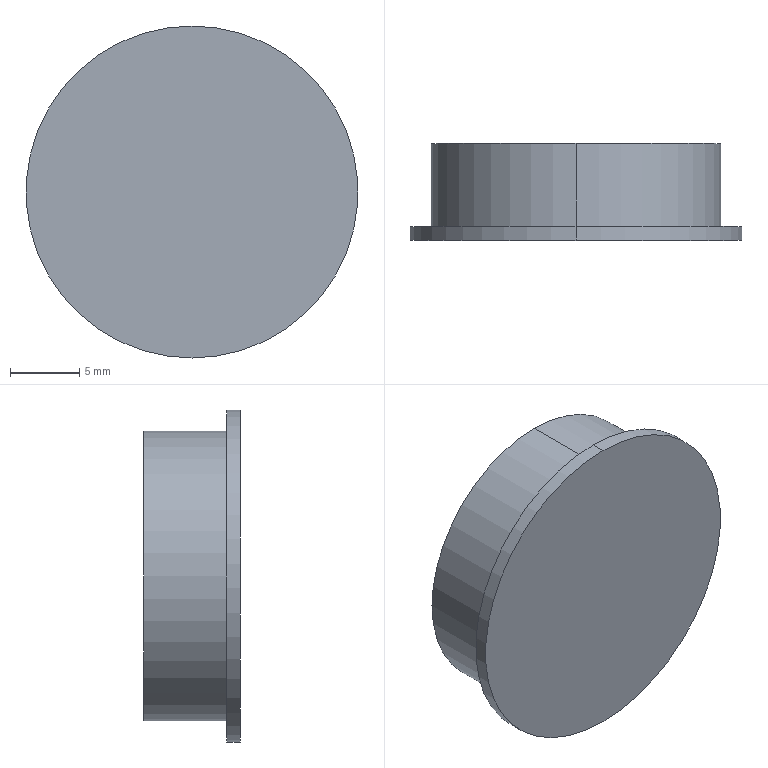Part | SolidWorks | features BaseBody 1 | 1 solid | 7 faces | box 24 x 7 x 24 mm | volume 2522 mm3 | cylinder 4 | plane 3 | commonest cylinder face diameters 20.955 x2 24 x2
STEP:
#1=CARTESIAN_POINT('',(0.,-1.,-12.));
#2=VERTEX_POINT('',#1);
#3=CARTESIAN_POINT('',(0.,-1.,12.));
#4=VERTEX_POINT('',#3);
#5=CARTESIAN_POINT('',(0.,-1.,0.));
#6=DIRECTION('',(0.,-1.,0.));
#7=DIRECTION('',(0.,0.,-1.));
#8=AXIS2_PLACEMENT_3D('',#5,#6,#7);
#9=CIRCLE('',#8,12.);
#10=EDGE_CURVE('',#2,#4,#9,.T.);
#11=ORIENTED_EDGE('',*,*,#10,.F.);
#12=CARTESIAN_POINT('',(0.,0.,-12.));
#13=VERTEX_POINT('',#12);
#14=CARTESIAN_POINT('',(0.,-1.,-12.));
#15=DIRECTION('',(0.,1.,0.));
#16=VECTOR('',#15,1000.);
#17=LINE('',#14,#16);
#18=EDGE_CURVE('',#2,#13,#17,.T.);
#19=ORIENTED_EDGE('',*,*,#18,.T.);
#20=CARTESIAN_POINT('',(0.,0.,12.));
#21=VERTEX_POINT('',#20);
#22=CARTESIAN_POINT('',(0.,0.,0.));
#23=DIRECTION('',(0.,-1.,0.));
#24=DIRECTION('',(0.,0.,-1.));
#25=AXIS2_PLACEMENT_3D('',#22,#23,#24);
#26=CIRCLE('',#25,12.);
#27=EDGE_CURVE('',#13,#21,#26,.T.);
#28=ORIENTED_EDGE('',*,*,#27,.T.);
#29=CARTESIAN_POINT('',(0.,-1.,12.));
#30=DIRECTION('',(0.,1.,0.));
#31=VECTOR('',#30,1000.);
#32=LINE('',#29,#31);
#33=EDGE_CURVE('',#4,#21,#32,.T.);
#34=ORIENTED_EDGE('',*,*,#33,.F.);
#35=EDGE_LOOP('',(#11,#19,#28,#34));
#36=FACE_OUTER_BOUND('',#35,.T.);
#37=CARTESIAN_POINT('',(0.,-1.,0.));
#38=DIRECTION('',(0.,1.,0.));
#39=DIRECTION('',(0.,0.,1.));
#40=AXIS2_PLACEMENT_3D('',#37,#38,#39);
#41=CYLINDRICAL_SURFACE('',#40,12.);
#42=ADVANCED_FACE('',(#36),#41,.T.);
#43=CARTESIAN_POINT('',(0.,6.,10.478));
#44=VERTEX_POINT('',#43);
#45=CARTESIAN_POINT('',(0.,6.,-10.478));
#46=VERTEX_POINT('',#45);
#47=CARTESIAN_POINT('',(0.,6.,0.));
#48=DIRECTION('',(0.,1.,0.));
#49=DIRECTION('',(0.,0.,1.));
#50=AXIS2_PLACEMENT_3D('',#47,#48,#49);
#51=CIRCLE('',#50,10.478);
#52=EDGE_CURVE('',#44,#46,#51,.T.);
#53=ORIENTED_EDGE('',*,*,#52,.F.);
#54=CARTESIAN_POINT('',(0.,0.,10.478));
#55=VERTEX_POINT('',#54);
#56=CARTESIAN_POINT('',(0.,6.,10.478));
#57=DIRECTION('',(0.,-1.,0.));
#58=VECTOR('',#57,1000.);
#59=LINE('',#56,#58);
#60=EDGE_CURVE('',#44,#55,#59,.T.);
#61=ORIENTED_EDGE('',*,*,#60,.T.);
#62=CARTESIAN_POINT('',(0.,0.,-10.478));
#63=VERTEX_POINT('',#62);
#64=CARTESIAN_POINT('',(0.,0.,0.));
#65=DIRECTION('',(0.,-1.,0.));
#66=DIRECTION('',(0.,0.,-1.));
#67=AXIS2_PLACEMENT_3D('',#64,#65,#66);
#68=CIRCLE('',#67,10.478);
#69=EDGE_CURVE('',#63,#55,#68,.T.);
#70=ORIENTED_EDGE('',*,*,#69,.F.);
#71=CARTESIAN_POINT('',(0.,6.,-10.478));
#72=DIRECTION('',(0.,-1.,0.));
#73=VECTOR('',#72,1000.);
#74=LINE('',#71,#73);
#75=EDGE_CURVE('',#46,#63,#74,.T.);
#76=ORIENTED_EDGE('',*,*,#75,.F.);
#77=EDGE_LOOP('',(#53,#61,#70,#76));
#78=FACE_OUTER_BOUND('',#77,.T.);
#79=CARTESIAN_POINT('',(0.,6.,0.));
#80=DIRECTION('',(0.,-1.,0.));
#81=DIRECTION('',(0.,0.,-1.));
#82=AXIS2_PLACEMENT_3D('',#79,#80,#81);
#83=CYLINDRICAL_SURFACE('',#82,10.478);
#84=ADVANCED_FACE('',(#78),#83,.T.);
#85=ORIENTED_EDGE('',*,*,#60,.F.);
#86=CARTESIAN_POINT('',(0.,6.,0.));
#87=DIRECTION('',(0.,1.,0.));
#88=DIRECTION('',(0.,0.,1.));
#89=AXIS2_PLACEMENT_3D('',#86,#87,#88);
#90=CIRCLE('',#89,10.478);
#91=EDGE_CURVE('',#46,#44,#90,.T.);
#92=ORIENTED_EDGE('',*,*,#91,.F.);
#93=ORIENTED_EDGE('',*,*,#75,.T.);
#94=CARTESIAN_POINT('',(0.,0.,0.));
#95=DIRECTION('',(0.,-1.,0.));
#96=DIRECTION('',(0.,0.,-1.));
#97=AXIS2_PLACEMENT_3D('',#94,#95,#96);
#98=CIRCLE('',#97,10.478);
#99=EDGE_CURVE('',#55,#63,#98,.T.);
#100=ORIENTED_EDGE('',*,*,#99,.F.);
#101=EDGE_LOOP('',(#85,#92,#93,#100));
#102=FACE_OUTER_BOUND('',#101,.T.);
#103=CARTESIAN_POINT('',(0.,6.,0.));
#104=DIRECTION('',(0.,-1.,0.));
#105=DIRECTION('',(0.,0.,-1.));
#106=AXIS2_PLACEMENT_3D('',#103,#104,#105);
#107=CYLINDRICAL_SURFACE('',#106,10.478);
#108=ADVANCED_FACE('',(#102),#107,.T.);
#109=ORIENTED_EDGE('',*,*,#91,.T.);
#110=ORIENTED_EDGE('',*,*,#52,.T.);
#111=EDGE_LOOP('',(#109,#110));
#112=FACE_OUTER_BOUND('',#111,.T.);
#113=CARTESIAN_POINT('',(0.,6.,0.));
#114=DIRECTION('',(0.,1.,0.));
#115=DIRECTION('',(0.,0.,1.));
#116=AXIS2_PLACEMENT_3D('',#113,#114,#115);
#117=PLANE('',#116);
#118=ADVANCED_FACE('',(#112),#117,.T.);
#119=CARTESIAN_POINT('',(0.,0.,0.));
#120=DIRECTION('',(0.,-1.,0.));
#121=DIRECTION('',(0.,0.,-1.));
#122=AXIS2_PLACEMENT_3D('',#119,#120,#121);
#123=CIRCLE('',#122,12.);
#124=EDGE_CURVE('',#21,#13,#123,.T.);
#125=ORIENTED_EDGE('',*,*,#124,.F.);
#126=ORIENTED_EDGE('',*,*,#27,.F.);
#127=EDGE_LOOP('',(#125,#126));
#128=FACE_OUTER_BOUND('',#127,.T.);
#129=ORIENTED_EDGE('',*,*,#69,.T.);
#130=ORIENTED_EDGE('',*,*,#99,.T.);
#131=EDGE_LOOP('',(#129,#130));
#132=FACE_BOUND('',#131,.T.);
#133=CARTESIAN_POINT('',(0.,0.,0.));
#134=DIRECTION('',(0.,-1.,0.));
#135=DIRECTION('',(0.,0.,-1.));
#136=AXIS2_PLACEMENT_3D('',#133,#134,#135);
#137=PLANE('',#136);
#138=ADVANCED_FACE('',(#128,#132),#137,.F.);
#139=ORIENTED_EDGE('',*,*,#18,.F.);
#140=CARTESIAN_POINT('',(0.,-1.,0.));
#141=DIRECTION('',(0.,-1.,0.));
#142=DIRECTION('',(0.,0.,-1.));
#143=AXIS2_PLACEMENT_3D('',#140,#141,#142);
#144=CIRCLE('',#143,12.);
#145=EDGE_CURVE('',#4,#2,#144,.T.);
#146=ORIENTED_EDGE('',*,*,#145,.F.);
#147=ORIENTED_EDGE('',*,*,#33,.T.);
#148=ORIENTED_EDGE('',*,*,#124,.T.);
#149=EDGE_LOOP('',(#139,#146,#147,#148));
#150=FACE_OUTER_BOUND('',#149,.T.);
#151=CARTESIAN_POINT('',(0.,-1.,0.));
#152=DIRECTION('',(0.,1.,0.));
#153=DIRECTION('',(0.,0.,1.));
#154=AXIS2_PLACEMENT_3D('',#151,#152,#153);
#155=CYLINDRICAL_SURFACE('',#154,12.);
#156=ADVANCED_FACE('',(#150),#155,.T.);
#157=ORIENTED_EDGE('',*,*,#145,.T.);
#158=ORIENTED_EDGE('',*,*,#10,.T.);
#159=EDGE_LOOP('',(#157,#158));
#160=FACE_OUTER_BOUND('',#159,.T.);
#161=CARTESIAN_POINT('',(0.,-1.,0.));
#162=DIRECTION('',(0.,-1.,0.));
#163=DIRECTION('',(0.,0.,-1.));
#164=AXIS2_PLACEMENT_3D('',#161,#162,#163);
#165=PLANE('',#164);
#166=ADVANCED_FACE('',(#160),#165,.T.);
#167=CLOSED_SHELL('',(#42,#84,#108,#118,#138,#156,#166));
#168=MANIFOLD_SOLID_BREP('',#167);
#169=CARTESIAN_POINT('',(0.,0.,0.));
#170=DIRECTION('',(0.,0.,1.));
#171=DIRECTION('',(1.,0.,0.));
#172=AXIS2_PLACEMENT_3D('',#169,#170,#171);
#173=(LENGTH_UNIT()NAMED_UNIT(*)SI_UNIT(.MILLI.,.METRE.));
#174=UNCERTAINTY_MEASURE_WITH_UNIT(LENGTH_MEASURE(0.00001),#173,'','');
#175=(NAMED_UNIT(*)PLANE_ANGLE_UNIT()SI_UNIT($,.RADIAN.));
#176=(NAMED_UNIT(*)SI_UNIT($,.STERADIAN.)SOLID_ANGLE_UNIT());
#177=(GEOMETRIC_REPRESENTATION_CONTEXT(3)GLOBAL_UNCERTAINTY_ASSIGNED_CONTEXT((#174))GLOBAL_UNIT_ASSIGNED_CONTEXT((#173,#175,#176))REPRESENTATION_CONTEXT('',''));
#178=ADVANCED_BREP_SHAPE_REPRESENTATION('',(#168,#172),#177);